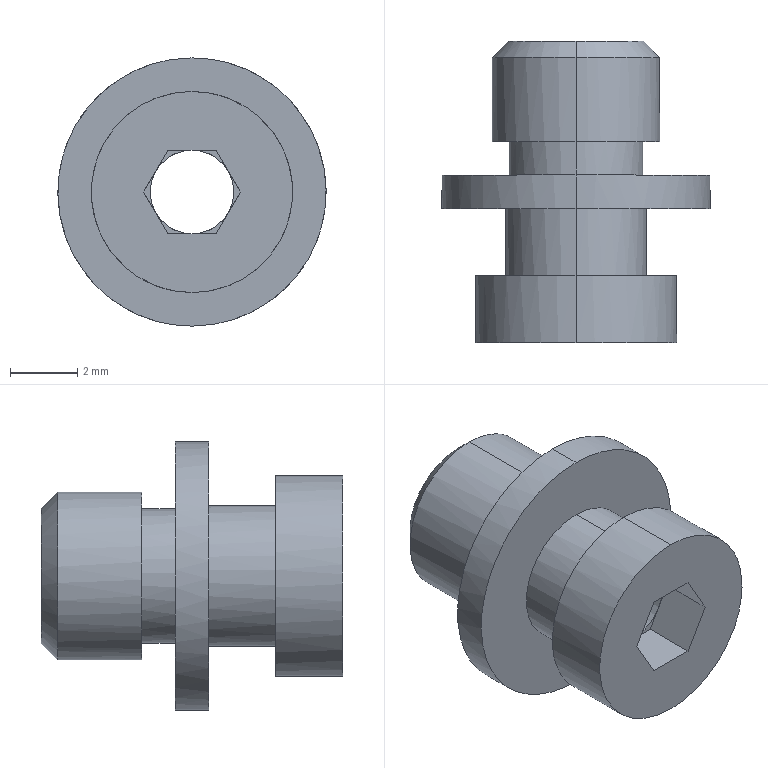Part | SolidWorks | features BaseBody 1 | 1 solid | 32 faces | box 8 x 9 x 8 mm | volume 159.238 mm3 | plane 18 | cylinder 12 | cone 2 | commonest cylinder face diameters 2.5 x2 4 x2 4.2 x2 5 x2 6 x2 8 x2
STEP:
#1=CARTESIAN_POINT('',(0.,0.,-2.1));
#2=VERTEX_POINT('',#1);
#3=CARTESIAN_POINT('',(0.,0.,2.1));
#4=VERTEX_POINT('',#3);
#5=CARTESIAN_POINT('',(0.,0.,-2.1));
#6=CARTESIAN_POINT('',(0.2749,0.,-2.1));
#7=CARTESIAN_POINT('',(0.5497,0.,-2.045));
#8=CARTESIAN_POINT('',(1.058,0.,-1.835));
#9=CARTESIAN_POINT('',(1.291,0.,-1.679));
#10=CARTESIAN_POINT('',(1.679,0.,-1.291));
#11=CARTESIAN_POINT('',(1.835,0.,-1.058));
#12=CARTESIAN_POINT('',(2.045,0.,-0.5497));
#13=CARTESIAN_POINT('',(2.1,0.,-0.2749));
#14=CARTESIAN_POINT('',(2.1,0.,0.2749));
#15=CARTESIAN_POINT('',(2.045,0.,0.5497));
#16=CARTESIAN_POINT('',(1.835,0.,1.058));
#17=CARTESIAN_POINT('',(1.679,0.,1.291));
#18=CARTESIAN_POINT('',(1.291,0.,1.679));
#19=CARTESIAN_POINT('',(1.058,0.,1.835));
#20=CARTESIAN_POINT('',(0.5497,0.,2.045));
#21=CARTESIAN_POINT('',(0.2749,0.,2.1));
#22=CARTESIAN_POINT('',(0.,0.,2.1));
#23=B_SPLINE_CURVE_WITH_KNOTS('',3,(#5,#6,#7,#8,#9,#10,#11,#12,#13,#14,#15,#16,#17,#18,#19,#20,#21,#22),.UNSPECIFIED.,.F.,.F.,(4,2,2,2,2,2,2,2,4),(0.,0.3927,0.7854,1.178,1.571,1.963,2.356,2.749,3.142),.UNSPECIFIED.);
#24=EDGE_CURVE('',#2,#4,#23,.T.);
#25=ORIENTED_EDGE('',*,*,#24,.T.);
#26=CARTESIAN_POINT('',(0.,-2.,2.1));
#27=VERTEX_POINT('',#26);
#28=CARTESIAN_POINT('',(0.,-4.,2.1));
#29=DIRECTION('',(0.,-1.,0.));
#30=VECTOR('',#29,1000.);
#31=LINE('',#28,#30);
#32=EDGE_CURVE('',#4,#27,#31,.T.);
#33=ORIENTED_EDGE('',*,*,#32,.T.);
#34=CARTESIAN_POINT('',(0.,-2.,-2.1));
#35=VERTEX_POINT('',#34);
#36=CARTESIAN_POINT('',(0.,-2.,-2.1));
#37=CARTESIAN_POINT('',(0.2785,-2.,-2.1));
#38=CARTESIAN_POINT('',(0.5464,-2.,-2.047));
#39=CARTESIAN_POINT('',(1.061,-2.,-1.834));
#40=CARTESIAN_POINT('',(1.288,-2.,-1.682));
#41=CARTESIAN_POINT('',(1.682,-2.,-1.288));
#42=CARTESIAN_POINT('',(1.834,-2.,-1.061));
#43=CARTESIAN_POINT('',(2.047,-2.,-0.5464));
#44=CARTESIAN_POINT('',(2.1,-2.,-0.2785));
#45=CARTESIAN_POINT('',(2.1,-2.,0.2785));
#46=CARTESIAN_POINT('',(2.047,-2.,0.5464));
#47=CARTESIAN_POINT('',(1.834,-2.,1.061));
#48=CARTESIAN_POINT('',(1.682,-2.,1.288));
#49=CARTESIAN_POINT('',(1.288,-2.,1.682));
#50=CARTESIAN_POINT('',(1.061,-2.,1.834));
#51=CARTESIAN_POINT('',(0.5464,-2.,2.047));
#52=CARTESIAN_POINT('',(0.2785,-2.,2.1));
#53=CARTESIAN_POINT('',(0.,-2.,2.1));
#54=B_SPLINE_CURVE_WITH_KNOTS('',3,(#36,#37,#38,#39,#40,#41,#42,#43,#44,#45,#46,#47,#48,#49,#50,#51,#52,#53),.UNSPECIFIED.,.F.,.F.,(4,2,2,2,2,2,2,2,4),(0.,0.3927,0.7854,1.178,1.571,1.963,2.356,2.749,3.142),.UNSPECIFIED.);
#55=EDGE_CURVE('',#35,#27,#54,.T.);
#56=ORIENTED_EDGE('',*,*,#55,.F.);
#57=CARTESIAN_POINT('',(0.,-4.,-2.1));
#58=DIRECTION('',(0.,-1.,0.));
#59=VECTOR('',#58,1000.);
#60=LINE('',#57,#59);
#61=EDGE_CURVE('',#2,#35,#60,.T.);
#62=ORIENTED_EDGE('',*,*,#61,.F.);
#63=EDGE_LOOP('',(#25,#33,#56,#62));
#64=FACE_OUTER_BOUND('',#63,.T.);
#65=CARTESIAN_POINT('',(0.,-4.,0.));
#66=DIRECTION('',(0.,-1.,0.));
#67=DIRECTION('',(0.,0.,-1.));
#68=AXIS2_PLACEMENT_3D('',#65,#66,#67);
#69=CYLINDRICAL_SURFACE('',#68,2.1);
#70=ADVANCED_FACE('',(#64),#69,.T.);
#71=CARTESIAN_POINT('',(0.,-2.,-3.));
#72=VERTEX_POINT('',#71);
#73=CARTESIAN_POINT('',(0.,-2.,3.));
#74=VERTEX_POINT('',#73);
#75=CARTESIAN_POINT('',(0.,-2.,-3.));
#76=CARTESIAN_POINT('',(0.3927,-2.,-3.));
#77=CARTESIAN_POINT('',(0.7852,-2.,-2.922));
#78=CARTESIAN_POINT('',(1.511,-2.,-2.621));
#79=CARTESIAN_POINT('',(1.844,-2.,-2.399));
#80=CARTESIAN_POINT('',(2.399,-2.,-1.844));
#81=CARTESIAN_POINT('',(2.621,-2.,-1.511));
#82=CARTESIAN_POINT('',(2.922,-2.,-0.7852));
#83=CARTESIAN_POINT('',(3.,-2.,-0.3927));
#84=CARTESIAN_POINT('',(3.,-2.,0.3927));
#85=CARTESIAN_POINT('',(2.922,-2.,0.7852));
#86=CARTESIAN_POINT('',(2.621,-2.,1.511));
#87=CARTESIAN_POINT('',(2.399,-2.,1.844));
#88=CARTESIAN_POINT('',(1.844,-2.,2.399));
#89=CARTESIAN_POINT('',(1.511,-2.,2.621));
#90=CARTESIAN_POINT('',(0.7852,-2.,2.922));
#91=CARTESIAN_POINT('',(0.3927,-2.,3.));
#92=CARTESIAN_POINT('',(0.,-2.,3.));
#93=B_SPLINE_CURVE_WITH_KNOTS('',3,(#75,#76,#77,#78,#79,#80,#81,#82,#83,#84,#85,#86,#87,#88,#89,#90,#91,#92),.UNSPECIFIED.,.F.,.F.,(4,2,2,2,2,2,2,2,4),(0.,0.3927,0.7854,1.178,1.571,1.963,2.356,2.749,3.142),.UNSPECIFIED.);
#94=EDGE_CURVE('',#72,#74,#93,.T.);
#95=ORIENTED_EDGE('',*,*,#94,.T.);
#96=CARTESIAN_POINT('',(0.,-4.,3.));
#97=VERTEX_POINT('',#96);
#98=CARTESIAN_POINT('',(0.,-4.,3.));
#99=DIRECTION('',(0.,-1.,0.));
#100=VECTOR('',#99,1000.);
#101=LINE('',#98,#100);
#102=EDGE_CURVE('',#74,#97,#101,.T.);
#103=ORIENTED_EDGE('',*,*,#102,.T.);
#104=CARTESIAN_POINT('',(0.,-4.,-3.));
#105=VERTEX_POINT('',#104);
#106=CARTESIAN_POINT('',(0.,-4.,-3.));
#107=CARTESIAN_POINT('',(0.3978,-4.,-3.));
#108=CARTESIAN_POINT('',(0.7805,-4.,-2.924));
#109=CARTESIAN_POINT('',(1.516,-4.,-2.619));
#110=CARTESIAN_POINT('',(1.84,-4.,-2.403));
#111=CARTESIAN_POINT('',(2.403,-4.,-1.84));
#112=CARTESIAN_POINT('',(2.619,-4.,-1.516));
#113=CARTESIAN_POINT('',(2.924,-4.,-0.7805));
#114=CARTESIAN_POINT('',(3.,-4.,-0.3978));
#115=CARTESIAN_POINT('',(3.,-4.,0.3978));
#116=CARTESIAN_POINT('',(2.924,-4.,0.7805));
#117=CARTESIAN_POINT('',(2.619,-4.,1.516));
#118=CARTESIAN_POINT('',(2.403,-4.,1.84));
#119=CARTESIAN_POINT('',(1.84,-4.,2.403));
#120=CARTESIAN_POINT('',(1.516,-4.,2.619));
#121=CARTESIAN_POINT('',(0.7805,-4.,2.924));
#122=CARTESIAN_POINT('',(0.3978,-4.,3.));
#123=CARTESIAN_POINT('',(0.,-4.,3.));
#124=B_SPLINE_CURVE_WITH_KNOTS('',3,(#106,#107,#108,#109,#110,#111,#112,#113,#114,#115,#116,#117,#118,#119,#120,#121,#122,#123),.UNSPECIFIED.,.F.,.F.,(4,2,2,2,2,2,2,2,4),(0.,0.3927,0.7854,1.178,1.571,1.963,2.356,2.749,3.142),.UNSPECIFIED.);
#125=EDGE_CURVE('',#105,#97,#124,.T.);
#126=ORIENTED_EDGE('',*,*,#125,.F.);
#127=CARTESIAN_POINT('',(0.,-4.,-3.));
#128=DIRECTION('',(0.,-1.,0.));
#129=VECTOR('',#128,1000.);
#130=LINE('',#127,#129);
#131=EDGE_CURVE('',#72,#105,#130,.T.);
#132=ORIENTED_EDGE('',*,*,#131,.F.);
#133=EDGE_LOOP('',(#95,#103,#126,#132));
#134=FACE_OUTER_BOUND('',#133,.T.);
#135=CARTESIAN_POINT('',(0.,-4.,0.));
#136=DIRECTION('',(0.,-1.,0.));
#137=DIRECTION('',(0.,0.,-1.));
#138=AXIS2_PLACEMENT_3D('',#135,#136,#137);
#139=CYLINDRICAL_SURFACE('',#138,3.);
#140=ADVANCED_FACE('',(#134),#139,.T.);
#141=CARTESIAN_POINT('',(0.,5.,-2.009));
#142=VERTEX_POINT('',#141);
#143=CARTESIAN_POINT('',(0.,5.,2.009));
#144=VERTEX_POINT('',#143);
#145=CARTESIAN_POINT('',(0.,5.,-2.009));
#146=CARTESIAN_POINT('',(0.263,5.,-2.009));
#147=CARTESIAN_POINT('',(0.526,5.,-1.957));
#148=CARTESIAN_POINT('',(1.012,5.,-1.756));
#149=CARTESIAN_POINT('',(1.235,5.,-1.607));
#150=CARTESIAN_POINT('',(1.607,5.,-1.235));
#151=CARTESIAN_POINT('',(1.756,5.,-1.012));
#152=CARTESIAN_POINT('',(1.957,5.,-0.526));
#153=CARTESIAN_POINT('',(2.009,5.,-0.263));
#154=CARTESIAN_POINT('',(2.009,5.,0.263));
#155=CARTESIAN_POINT('',(1.957,5.,0.526));
#156=CARTESIAN_POINT('',(1.756,5.,1.012));
#157=CARTESIAN_POINT('',(1.607,5.,1.235));
#158=CARTESIAN_POINT('',(1.235,5.,1.607));
#159=CARTESIAN_POINT('',(1.012,5.,1.756));
#160=CARTESIAN_POINT('',(0.526,5.,1.957));
#161=CARTESIAN_POINT('',(0.263,5.,2.009));
#162=CARTESIAN_POINT('',(0.,5.,2.009));
#163=B_SPLINE_CURVE_WITH_KNOTS('',3,(#145,#146,#147,#148,#149,#150,#151,#152,#153,#154,#155,#156,#157,#158,#159,#160,#161,#162),.UNSPECIFIED.,.F.,.F.,(4,2,2,2,2,2,2,2,4),(0.,0.3927,0.7854,1.178,1.571,1.963,2.356,2.749,3.142),.UNSPECIFIED.);
#164=EDGE_CURVE('',#142,#144,#163,.T.);
#165=ORIENTED_EDGE('',*,*,#164,.T.);
#166=CARTESIAN_POINT('',(0.,4.509,2.5));
#167=VERTEX_POINT('',#166);
#168=CARTESIAN_POINT('',(0.,4.509,2.5));
#169=DIRECTION('',(0.,-0.7071,0.7071));
#170=VECTOR('',#169,1000.);
#171=LINE('',#168,#170);
#172=EDGE_CURVE('',#144,#167,#171,.T.);
#173=ORIENTED_EDGE('',*,*,#172,.T.);
#174=CARTESIAN_POINT('',(0.,4.509,-2.5));
#175=VERTEX_POINT('',#174);
#176=CARTESIAN_POINT('',(0.,4.509,-2.5));
#177=CARTESIAN_POINT('',(0.3272,4.509,-2.5));
#178=CARTESIAN_POINT('',(0.6544,4.509,-2.435));
#179=CARTESIAN_POINT('',(1.259,4.509,-2.184));
#180=CARTESIAN_POINT('',(1.536,4.51,-1.999));
#181=CARTESIAN_POINT('',(1.999,4.509,-1.536));
#182=CARTESIAN_POINT('',(2.184,4.51,-1.259));
#183=CARTESIAN_POINT('',(2.435,4.509,-0.6544));
#184=CARTESIAN_POINT('',(2.5,4.51,-0.3272));
#185=CARTESIAN_POINT('',(2.5,4.509,0.3272));
#186=CARTESIAN_POINT('',(2.435,4.509,0.6544));
#187=CARTESIAN_POINT('',(2.184,4.509,1.259));
#188=CARTESIAN_POINT('',(1.999,4.509,1.536));
#189=CARTESIAN_POINT('',(1.536,4.509,1.999));
#190=CARTESIAN_POINT('',(1.259,4.509,2.184));
#191=CARTESIAN_POINT('',(0.6544,4.51,2.435));
#192=CARTESIAN_POINT('',(0.3272,4.51,2.5));
#193=CARTESIAN_POINT('',(0.,4.509,2.5));
#194=B_SPLINE_CURVE_WITH_KNOTS('',3,(#176,#177,#178,#179,#180,#181,#182,#183,#184,#185,#186,#187,#188,#189,#190,#191,#192,#193),.UNSPECIFIED.,.F.,.F.,(4,2,2,2,2,2,2,2,4),(0.,0.3927,0.7854,1.178,1.571,1.963,2.356,2.749,3.142),.UNSPECIFIED.);
#195=EDGE_CURVE('',#175,#167,#194,.T.);
#196=ORIENTED_EDGE('',*,*,#195,.F.);
#197=CARTESIAN_POINT('',(0.,4.509,-2.5));
#198=DIRECTION('',(0.,-0.7071,-0.7071));
#199=VECTOR('',#198,1000.);
#200=LINE('',#197,#199);
#201=EDGE_CURVE('',#142,#175,#200,.T.);
#202=ORIENTED_EDGE('',*,*,#201,.F.);
#203=EDGE_LOOP('',(#165,#173,#196,#202));
#204=FACE_OUTER_BOUND('',#203,.T.);
#205=CARTESIAN_POINT('',(0.,4.509,0.));
#206=DIRECTION('',(0.,-1.,0.));
#207=DIRECTION('',(0.,0.,-1.));
#208=AXIS2_PLACEMENT_3D('',#205,#206,#207);
#209=CONICAL_SURFACE('',#208,2.5,0.7854);
#210=ADVANCED_FACE('',(#204),#209,.T.);
#211=ORIENTED_EDGE('',*,*,#195,.T.);
#212=CARTESIAN_POINT('',(0.,2.,2.5));
#213=VERTEX_POINT('',#212);
#214=CARTESIAN_POINT('',(0.,0.,2.5));
#215=DIRECTION('',(0.,-1.,0.));
#216=VECTOR('',#215,1000.);
#217=LINE('',#214,#216);
#218=EDGE_CURVE('',#167,#213,#217,.T.);
#219=ORIENTED_EDGE('',*,*,#218,.T.);
#220=CARTESIAN_POINT('',(0.,2.,-2.5));
#221=VERTEX_POINT('',#220);
#222=CARTESIAN_POINT('',(0.,2.,-2.5));
#223=CARTESIAN_POINT('',(0.3315,2.,-2.5));
#224=CARTESIAN_POINT('',(0.6504,2.,-2.437));
#225=CARTESIAN_POINT('',(1.263,2.,-2.183));
#226=CARTESIAN_POINT('',(1.533,2.,-2.002));
#227=CARTESIAN_POINT('',(2.002,2.,-1.533));
#228=CARTESIAN_POINT('',(2.183,2.,-1.263));
#229=CARTESIAN_POINT('',(2.437,2.,-0.6504));
#230=CARTESIAN_POINT('',(2.5,2.,-0.3315));
#231=CARTESIAN_POINT('',(2.5,2.,0.3315));
#232=CARTESIAN_POINT('',(2.437,2.,0.6504));
#233=CARTESIAN_POINT('',(2.183,2.,1.263));
#234=CARTESIAN_POINT('',(2.002,2.,1.533));
#235=CARTESIAN_POINT('',(1.533,2.,2.002));
#236=CARTESIAN_POINT('',(1.263,2.,2.183));
#237=CARTESIAN_POINT('',(0.6504,2.,2.437));
#238=CARTESIAN_POINT('',(0.3315,2.,2.5));
#239=CARTESIAN_POINT('',(0.,2.,2.5));
#240=B_SPLINE_CURVE_WITH_KNOTS('',3,(#222,#223,#224,#225,#226,#227,#228,#229,#230,#231,#232,#233,#234,#235,#236,#237,#238,#239),.UNSPECIFIED.,.F.,.F.,(4,2,2,2,2,2,2,2,4),(0.,0.3927,0.7854,1.178,1.571,1.963,2.356,2.749,3.142),.UNSPECIFIED.);
#241=EDGE_CURVE('',#221,#213,#240,.T.);
#242=ORIENTED_EDGE('',*,*,#241,.F.);
#243=CARTESIAN_POINT('',(0.,0.,-2.5));
#244=DIRECTION('',(0.,-1.,0.));
#245=VECTOR('',#244,1000.);
#246=LINE('',#243,#245);
#247=EDGE_CURVE('',#175,#221,#246,.T.);
#248=ORIENTED_EDGE('',*,*,#247,.F.);
#249=EDGE_LOOP('',(#211,#219,#242,#248));
#250=FACE_OUTER_BOUND('',#249,.T.);
#251=CARTESIAN_POINT('',(0.,0.,0.));
#252=DIRECTION('',(0.,-1.,0.));
#253=DIRECTION('',(0.,0.,-1.));
#254=AXIS2_PLACEMENT_3D('',#251,#252,#253);
#255=CYLINDRICAL_SURFACE('',#254,2.5);
#256=ADVANCED_FACE('',(#250),#255,.T.);
#257=CARTESIAN_POINT('',(0.,2.,-2.));
#258=VERTEX_POINT('',#257);
#259=CARTESIAN_POINT('',(0.,2.,2.));
#260=VERTEX_POINT('',#259);
#261=CARTESIAN_POINT('',(0.,2.,-2.));
#262=CARTESIAN_POINT('',(0.2618,2.,-2.));
#263=CARTESIAN_POINT('',(0.5235,2.,-1.948));
#264=CARTESIAN_POINT('',(1.007,2.,-1.748));
#265=CARTESIAN_POINT('',(1.229,2.,-1.599));
#266=CARTESIAN_POINT('',(1.599,2.,-1.229));
#267=CARTESIAN_POINT('',(1.748,2.,-1.007));
#268=CARTESIAN_POINT('',(1.948,2.,-0.5235));
#269=CARTESIAN_POINT('',(2.,2.,-0.2618));
#270=CARTESIAN_POINT('',(2.,2.,0.2618));
#271=CARTESIAN_POINT('',(1.948,2.,0.5235));
#272=CARTESIAN_POINT('',(1.748,2.,1.007));
#273=CARTESIAN_POINT('',(1.599,2.,1.229));
#274=CARTESIAN_POINT('',(1.229,2.,1.599));
#275=CARTESIAN_POINT('',(1.007,2.,1.748));
#276=CARTESIAN_POINT('',(0.5235,2.,1.948));
#277=CARTESIAN_POINT('',(0.2618,2.,2.));
#278=CARTESIAN_POINT('',(0.,2.,2.));
#279=B_SPLINE_CURVE_WITH_KNOTS('',3,(#261,#262,#263,#264,#265,#266,#267,#268,#269,#270,#271,#272,#273,#274,#275,#276,#277,#278),.UNSPECIFIED.,.F.,.F.,(4,2,2,2,2,2,2,2,4),(0.,0.3927,0.7854,1.178,1.571,1.963,2.356,2.749,3.142),.UNSPECIFIED.);
#280=EDGE_CURVE('',#258,#260,#279,.T.);
#281=ORIENTED_EDGE('',*,*,#280,.T.);
#282=CARTESIAN_POINT('',(0.,1.,2.));
#283=VERTEX_POINT('',#282);
#284=CARTESIAN_POINT('',(0.,0.,2.));
#285=DIRECTION('',(0.,-1.,0.));
#286=VECTOR('',#285,1000.);
#287=LINE('',#284,#286);
#288=EDGE_CURVE('',#260,#283,#287,.T.);
#289=ORIENTED_EDGE('',*,*,#288,.T.);
#290=CARTESIAN_POINT('',(0.,1.,-2.));
#291=VERTEX_POINT('',#290);
#292=CARTESIAN_POINT('',(0.,1.,-2.));
#293=CARTESIAN_POINT('',(0.2652,1.,-2.));
#294=CARTESIAN_POINT('',(0.5203,1.,-1.949));
#295=CARTESIAN_POINT('',(1.01,1.,-1.746));
#296=CARTESIAN_POINT('',(1.227,1.,-1.602));
#297=CARTESIAN_POINT('',(1.602,1.,-1.227));
#298=CARTESIAN_POINT('',(1.746,1.,-1.01));
#299=CARTESIAN_POINT('',(1.949,1.,-0.5203));
#300=CARTESIAN_POINT('',(2.,1.,-0.2652));
#301=CARTESIAN_POINT('',(2.,1.,0.2652));
#302=CARTESIAN_POINT('',(1.949,1.,0.5203));
#303=CARTESIAN_POINT('',(1.746,1.,1.01));
#304=CARTESIAN_POINT('',(1.602,1.,1.227));
#305=CARTESIAN_POINT('',(1.227,1.,1.602));
#306=CARTESIAN_POINT('',(1.01,1.,1.746));
#307=CARTESIAN_POINT('',(0.5203,1.,1.949));
#308=CARTESIAN_POINT('',(0.2652,1.,2.));
#309=CARTESIAN_POINT('',(0.,1.,2.));
#310=B_SPLINE_CURVE_WITH_KNOTS('',3,(#292,#293,#294,#295,#296,#297,#298,#299,#300,#301,#302,#303,#304,#305,#306,#307,#308,#309),.UNSPECIFIED.,.F.,.F.,(4,2,2,2,2,2,2,2,4),(0.,0.3927,0.7854,1.178,1.571,1.963,2.356,2.749,3.142),.UNSPECIFIED.);
#311=EDGE_CURVE('',#291,#283,#310,.T.);
#312=ORIENTED_EDGE('',*,*,#311,.F.);
#313=CARTESIAN_POINT('',(0.,0.,-2.));
#314=DIRECTION('',(0.,-1.,0.));
#315=VECTOR('',#314,1000.);
#316=LINE('',#313,#315);
#317=EDGE_CURVE('',#258,#291,#316,.T.);
#318=ORIENTED_EDGE('',*,*,#317,.F.);
#319=EDGE_LOOP('',(#281,#289,#312,#318));
#320=FACE_OUTER_BOUND('',#319,.T.);
#321=CARTESIAN_POINT('',(0.,0.,0.));
#322=DIRECTION('',(0.,-1.,0.));
#323=DIRECTION('',(0.,0.,-1.));
#324=AXIS2_PLACEMENT_3D('',#321,#322,#323);
#325=CYLINDRICAL_SURFACE('',#324,2.);
#326=ADVANCED_FACE('',(#320),#325,.T.);
#327=CARTESIAN_POINT('',(0.,1.,-4.));
#328=VERTEX_POINT('',#327);
#329=CARTESIAN_POINT('',(0.,1.,4.));
#330=VERTEX_POINT('',#329);
#331=CARTESIAN_POINT('',(0.,1.,-4.));
#332=CARTESIAN_POINT('',(0.5236,1.,-4.));
#333=CARTESIAN_POINT('',(1.047,1.,-3.896));
#334=CARTESIAN_POINT('',(2.014,1.,-3.495));
#335=CARTESIAN_POINT('',(2.458,1.,-3.199));
#336=CARTESIAN_POINT('',(3.199,1.,-2.458));
#337=CARTESIAN_POINT('',(3.495,1.,-2.014));
#338=CARTESIAN_POINT('',(3.896,1.,-1.047));
#339=CARTESIAN_POINT('',(4.,1.,-0.5236));
#340=CARTESIAN_POINT('',(4.,1.,0.5236));
#341=CARTESIAN_POINT('',(3.896,1.,1.047));
#342=CARTESIAN_POINT('',(3.495,1.,2.014));
#343=CARTESIAN_POINT('',(3.199,1.,2.458));
#344=CARTESIAN_POINT('',(2.458,1.,3.199));
#345=CARTESIAN_POINT('',(2.014,1.,3.495));
#346=CARTESIAN_POINT('',(1.047,1.,3.896));
#347=CARTESIAN_POINT('',(0.5236,1.,4.));
#348=CARTESIAN_POINT('',(0.,1.,4.));
#349=B_SPLINE_CURVE_WITH_KNOTS('',3,(#331,#332,#333,#334,#335,#336,#337,#338,#339,#340,#341,#342,#343,#344,#345,#346,#347,#348),.UNSPECIFIED.,.F.,.F.,(4,2,2,2,2,2,2,2,4),(0.,0.3927,0.7854,1.178,1.571,1.963,2.356,2.749,3.142),.UNSPECIFIED.);
#350=EDGE_CURVE('',#328,#330,#349,.T.);
#351=ORIENTED_EDGE('',*,*,#350,.T.);
#352=CARTESIAN_POINT('',(0.,0.,4.));
#353=VERTEX_POINT('',#352);
#354=CARTESIAN_POINT('',(0.,0.,4.));
#355=DIRECTION('',(0.,-1.,0.));
#356=VECTOR('',#355,1000.);
#357=LINE('',#354,#356);
#358=EDGE_CURVE('',#330,#353,#357,.T.);
#359=ORIENTED_EDGE('',*,*,#358,.T.);
#360=CARTESIAN_POINT('',(0.,0.,-4.));
#361=VERTEX_POINT('',#360);
#362=CARTESIAN_POINT('',(0.,0.,-4.));
#363=CARTESIAN_POINT('',(0.5304,0.,-4.));
#364=CARTESIAN_POINT('',(1.041,0.,-3.899));
#365=CARTESIAN_POINT('',(2.021,0.,-3.493));
#366=CARTESIAN_POINT('',(2.453,0.,-3.203));
#367=CARTESIAN_POINT('',(3.203,0.,-2.453));
#368=CARTESIAN_POINT('',(3.493,0.,-2.021));
#369=CARTESIAN_POINT('',(3.899,0.,-1.041));
#370=CARTESIAN_POINT('',(4.,0.,-0.5304));
#371=CARTESIAN_POINT('',(4.,0.,0.5304));
#372=CARTESIAN_POINT('',(3.899,0.,1.041));
#373=CARTESIAN_POINT('',(3.493,0.,2.021));
#374=CARTESIAN_POINT('',(3.203,0.,2.453));
#375=CARTESIAN_POINT('',(2.453,0.,3.203));
#376=CARTESIAN_POINT('',(2.021,0.,3.493));
#377=CARTESIAN_POINT('',(1.041,0.,3.899));
#378=CARTESIAN_POINT('',(0.5304,0.,4.));
#379=CARTESIAN_POINT('',(0.,0.,4.));
#380=B_SPLINE_CURVE_WITH_KNOTS('',3,(#362,#363,#364,#365,#366,#367,#368,#369,#370,#371,#372,#373,#374,#375,#376,#377,#378,#379),.UNSPECIFIED.,.F.,.F.,(4,2,2,2,2,2,2,2,4),(0.,0.3927,0.7854,1.178,1.571,1.963,2.356,2.749,3.142),.UNSPECIFIED.);
#381=EDGE_CURVE('',#361,#353,#380,.T.);
#382=ORIENTED_EDGE('',*,*,#381,.F.);
#383=CARTESIAN_POINT('',(0.,0.,-4.));
#384=DIRECTION('',(0.,-1.,0.));
#385=VECTOR('',#384,1000.);
#386=LINE('',#383,#385);
#387=EDGE_CURVE('',#328,#361,#386,.T.);
#388=ORIENTED_EDGE('',*,*,#387,.F.);
#389=EDGE_LOOP('',(#351,#359,#382,#388));
#390=FACE_OUTER_BOUND('',#389,.T.);
#391=CARTESIAN_POINT('',(0.,0.,0.));
#392=DIRECTION('',(0.,-1.,0.));
#393=DIRECTION('',(0.,0.,-1.));
#394=AXIS2_PLACEMENT_3D('',#391,#392,#393);
#395=CYLINDRICAL_SURFACE('',#394,4.);
#396=ADVANCED_FACE('',(#390),#395,.T.);
#397=CARTESIAN_POINT('',(0.,5.,1.25));
#398=VERTEX_POINT('',#397);
#399=CARTESIAN_POINT('',(0.,5.,-1.25));
#400=VERTEX_POINT('',#399);
#401=CARTESIAN_POINT('',(0.,5.,1.25));
#402=CARTESIAN_POINT('',(-0.1658,5.,1.25));
#403=CARTESIAN_POINT('',(-0.3252,5.,1.218));
#404=CARTESIAN_POINT('',(-0.6315,5.,1.091));
#405=CARTESIAN_POINT('',(-0.7667,5.,1.001));
#406=CARTESIAN_POINT('',(-1.001,5.,0.7667));
#407=CARTESIAN_POINT('',(-1.091,5.,0.6315));
#408=CARTESIAN_POINT('',(-1.218,5.,0.3252));
#409=CARTESIAN_POINT('',(-1.25,5.,0.1658));
#410=CARTESIAN_POINT('',(-1.25,5.,-0.1658));
#411=CARTESIAN_POINT('',(-1.218,5.,-0.3252));
#412=CARTESIAN_POINT('',(-1.091,5.,-0.6315));
#413=CARTESIAN_POINT('',(-1.001,5.,-0.7667));
#414=CARTESIAN_POINT('',(-0.7667,5.,-1.001));
#415=CARTESIAN_POINT('',(-0.6315,5.,-1.091));
#416=CARTESIAN_POINT('',(-0.3252,5.,-1.218));
#417=CARTESIAN_POINT('',(-0.1658,5.,-1.25));
#418=CARTESIAN_POINT('',(0.,5.,-1.25));
#419=B_SPLINE_CURVE_WITH_KNOTS('',3,(#401,#402,#403,#404,#405,#406,#407,#408,#409,#410,#411,#412,#413,#414,#415,#416,#417,#418),.UNSPECIFIED.,.F.,.F.,(4,2,2,2,2,2,2,2,4),(3.142,3.534,3.927,4.32,4.712,5.105,5.498,5.89,6.283),.UNSPECIFIED.);
#420=EDGE_CURVE('',#398,#400,#419,.T.);
#421=ORIENTED_EDGE('',*,*,#420,.F.);
#422=CARTESIAN_POINT('',(0.,-2.4,1.25));
#423=VERTEX_POINT('',#422);
#424=CARTESIAN_POINT('',(0.,0.,1.25));
#425=DIRECTION('',(0.,-1.,0.));
#426=VECTOR('',#425,1000.);
#427=LINE('',#424,#426);
#428=EDGE_CURVE('',#398,#423,#427,.T.);
#429=ORIENTED_EDGE('',*,*,#428,.T.);
#430=CARTESIAN_POINT('',(-1.083,-2.4,0.625));
#431=VERTEX_POINT('',#430);
#432=CARTESIAN_POINT('',(0.,-2.4,0.));
#433=DIRECTION('',(0.,-1.,0.));
#434=DIRECTION('',(0.,0.,1.));
#435=AXIS2_PLACEMENT_3D('',#432,#433,#434);
#436=CIRCLE('',#435,1.25);
#437=EDGE_CURVE('',#423,#431,#436,.T.);
#438=ORIENTED_EDGE('',*,*,#437,.T.);
#439=CARTESIAN_POINT('',(-1.083,-2.4,-0.625));
#440=VERTEX_POINT('',#439);
#441=CARTESIAN_POINT('',(0.,-2.4,0.));
#442=DIRECTION('',(0.,-1.,0.));
#443=DIRECTION('',(-0.866,0.,0.5));
#444=AXIS2_PLACEMENT_3D('',#441,#442,#443);
#445=CIRCLE('',#444,1.25);
#446=EDGE_CURVE('',#431,#440,#445,.T.);
#447=ORIENTED_EDGE('',*,*,#446,.T.);
#448=CARTESIAN_POINT('',(0.,-2.4,-1.25));
#449=VERTEX_POINT('',#448);
#450=CARTESIAN_POINT('',(0.,-2.4,0.));
#451=DIRECTION('',(0.,-1.,0.));
#452=DIRECTION('',(-0.866,0.,-0.5));
#453=AXIS2_PLACEMENT_3D('',#450,#451,#452);
#454=CIRCLE('',#453,1.25);
#455=EDGE_CURVE('',#440,#449,#454,.T.);
#456=ORIENTED_EDGE('',*,*,#455,.T.);
#457=CARTESIAN_POINT('',(0.,0.,-1.25));
#458=DIRECTION('',(0.,-1.,0.));
#459=VECTOR('',#458,1000.);
#460=LINE('',#457,#459);
#461=EDGE_CURVE('',#400,#449,#460,.T.);
#462=ORIENTED_EDGE('',*,*,#461,.F.);
#463=EDGE_LOOP('',(#421,#429,#438,#447,#456,#462));
#464=FACE_OUTER_BOUND('',#463,.T.);
#465=CARTESIAN_POINT('',(0.,0.,0.));
#466=DIRECTION('',(0.,-1.,0.));
#467=DIRECTION('',(0.,0.,-1.));
#468=AXIS2_PLACEMENT_3D('',#465,#466,#467);
#469=CYLINDRICAL_SURFACE('',#468,1.25);
#470=ADVANCED_FACE('',(#464),#469,.F.);
#471=ORIENTED_EDGE('',*,*,#428,.F.);
#472=CARTESIAN_POINT('',(0.,5.,-1.25));
#473=CARTESIAN_POINT('',(0.1658,5.,-1.25));
#474=CARTESIAN_POINT('',(0.3252,5.,-1.218));
#475=CARTESIAN_POINT('',(0.6315,5.,-1.091));
#476=CARTESIAN_POINT('',(0.7667,5.,-1.001));
#477=CARTESIAN_POINT('',(1.001,5.,-0.7667));
#478=CARTESIAN_POINT('',(1.091,5.,-0.6315));
#479=CARTESIAN_POINT('',(1.218,5.,-0.3252));
#480=CARTESIAN_POINT('',(1.25,5.,-0.1658));
#481=CARTESIAN_POINT('',(1.25,5.,0.1658));
#482=CARTESIAN_POINT('',(1.218,5.,0.3252));
#483=CARTESIAN_POINT('',(1.091,5.,0.6315));
#484=CARTESIAN_POINT('',(1.001,5.,0.7667));
#485=CARTESIAN_POINT('',(0.7667,5.,1.001));
#486=CARTESIAN_POINT('',(0.6315,5.,1.091));
#487=CARTESIAN_POINT('',(0.3252,5.,1.218));
#488=CARTESIAN_POINT('',(0.1658,5.,1.25));
#489=CARTESIAN_POINT('',(0.,5.,1.25));
#490=B_SPLINE_CURVE_WITH_KNOTS('',3,(#472,#473,#474,#475,#476,#477,#478,#479,#480,#481,#482,#483,#484,#485,#486,#487,#488,#489),.UNSPECIFIED.,.F.,.F.,(4,2,2,2,2,2,2,2,4),(0.,0.3927,0.7854,1.178,1.571,1.963,2.356,2.749,3.142),.UNSPECIFIED.);
#491=EDGE_CURVE('',#400,#398,#490,.T.);
#492=ORIENTED_EDGE('',*,*,#491,.F.);
#493=ORIENTED_EDGE('',*,*,#461,.T.);
#494=CARTESIAN_POINT('',(1.083,-2.4,-0.625));
#495=VERTEX_POINT('',#494);
#496=CARTESIAN_POINT('',(0.,-2.4,0.));
#497=DIRECTION('',(0.,-1.,0.));
#498=DIRECTION('',(0.,0.,-1.));
#499=AXIS2_PLACEMENT_3D('',#496,#497,#498);
#500=CIRCLE('',#499,1.25);
#501=EDGE_CURVE('',#449,#495,#500,.T.);
#502=ORIENTED_EDGE('',*,*,#501,.T.);
#503=CARTESIAN_POINT('',(1.083,-2.4,0.625));
#504=VERTEX_POINT('',#503);
#505=CARTESIAN_POINT('',(0.,-2.4,0.));
#506=DIRECTION('',(0.,-1.,0.));
#507=DIRECTION('',(0.866,0.,-0.5));
#508=AXIS2_PLACEMENT_3D('',#505,#506,#507);
#509=CIRCLE('',#508,1.25);
#510=EDGE_CURVE('',#495,#504,#509,.T.);
#511=ORIENTED_EDGE('',*,*,#510,.T.);
#512=CARTESIAN_POINT('',(0.,-2.4,0.));
#513=DIRECTION('',(0.,-1.,0.));
#514=DIRECTION('',(0.866,0.,0.5));
#515=AXIS2_PLACEMENT_3D('',#512,#513,#514);
#516=CIRCLE('',#515,1.25);
#517=EDGE_CURVE('',#504,#423,#516,.T.);
#518=ORIENTED_EDGE('',*,*,#517,.T.);
#519=EDGE_LOOP('',(#471,#492,#493,#502,#511,#518));
#520=FACE_OUTER_BOUND('',#519,.T.);
#521=CARTESIAN_POINT('',(0.,0.,0.));
#522=DIRECTION('',(0.,-1.,0.));
#523=DIRECTION('',(0.,0.,-1.));
#524=AXIS2_PLACEMENT_3D('',#521,#522,#523);
#525=CYLINDRICAL_SURFACE('',#524,1.25);
#526=ADVANCED_FACE('',(#520),#525,.F.);
#527=ORIENTED_EDGE('',*,*,#491,.T.);
#528=ORIENTED_EDGE('',*,*,#420,.T.);
#529=EDGE_LOOP('',(#527,#528));
#530=FACE_BOUND('',#529,.T.);
#531=ORIENTED_EDGE('',*,*,#164,.F.);
#532=CARTESIAN_POINT('',(0.,5.,2.009));
#533=CARTESIAN_POINT('',(-0.263,5.,2.009));
#534=CARTESIAN_POINT('',(-0.526,5.,1.957));
#535=CARTESIAN_POINT('',(-1.012,5.,1.756));
#536=CARTESIAN_POINT('',(-1.235,5.,1.607));
#537=CARTESIAN_POINT('',(-1.607,5.,1.235));
#538=CARTESIAN_POINT('',(-1.756,5.,1.012));
#539=CARTESIAN_POINT('',(-1.957,5.,0.526));
#540=CARTESIAN_POINT('',(-2.009,5.,0.263));
#541=CARTESIAN_POINT('',(-2.009,5.,-0.263));
#542=CARTESIAN_POINT('',(-1.957,5.,-0.526));
#543=CARTESIAN_POINT('',(-1.756,5.,-1.012));
#544=CARTESIAN_POINT('',(-1.607,5.,-1.235));
#545=CARTESIAN_POINT('',(-1.235,5.,-1.607));
#546=CARTESIAN_POINT('',(-1.012,5.,-1.756));
#547=CARTESIAN_POINT('',(-0.526,5.,-1.957));
#548=CARTESIAN_POINT('',(-0.263,5.,-2.009));
#549=CARTESIAN_POINT('',(0.,5.,-2.009));
#550=B_SPLINE_CURVE_WITH_KNOTS('',3,(#532,#533,#534,#535,#536,#537,#538,#539,#540,#541,#542,#543,#544,#545,#546,#547,#548,#549),.UNSPECIFIED.,.F.,.F.,(4,2,2,2,2,2,2,2,4),(3.142,3.534,3.927,4.32,4.712,5.105,5.498,5.89,6.283),.UNSPECIFIED.);
#551=EDGE_CURVE('',#144,#142,#550,.T.);
#552=ORIENTED_EDGE('',*,*,#551,.F.);
#553=EDGE_LOOP('',(#531,#552));
#554=FACE_OUTER_BOUND('',#553,.T.);
#555=CARTESIAN_POINT('',(2.009,5.,0.));
#556=DIRECTION('',(0.,1.,0.));
#557=DIRECTION('',(0.,0.,1.));
#558=AXIS2_PLACEMENT_3D('',#555,#556,#557);
#559=PLANE('',#558);
#560=ADVANCED_FACE('',(#530,#554),#559,.T.);
#561=ORIENTED_EDGE('',*,*,#381,.T.);
#562=CARTESIAN_POINT('',(0.,0.,4.));
#563=CARTESIAN_POINT('',(-0.5304,0.,4.));
#564=CARTESIAN_POINT('',(-1.041,0.,3.899));
#565=CARTESIAN_POINT('',(-2.021,0.,3.493));
#566=CARTESIAN_POINT('',(-2.453,0.,3.203));
#567=CARTESIAN_POINT('',(-3.203,0.,2.453));
#568=CARTESIAN_POINT('',(-3.493,0.,2.021));
#569=CARTESIAN_POINT('',(-3.899,0.,1.041));
#570=CARTESIAN_POINT('',(-4.,0.,0.5304));
#571=CARTESIAN_POINT('',(-4.,0.,-0.5304));
#572=CARTESIAN_POINT('',(-3.899,0.,-1.041));
#573=CARTESIAN_POINT('',(-3.493,0.,-2.021));
#574=CARTESIAN_POINT('',(-3.203,0.,-2.453));
#575=CARTESIAN_POINT('',(-2.453,0.,-3.203));
#576=CARTESIAN_POINT('',(-2.021,0.,-3.493));
#577=CARTESIAN_POINT('',(-1.041,0.,-3.899));
#578=CARTESIAN_POINT('',(-0.5304,0.,-4.));
#579=CARTESIAN_POINT('',(0.,0.,-4.));
#580=B_SPLINE_CURVE_WITH_KNOTS('',3,(#562,#563,#564,#565,#566,#567,#568,#569,#570,#571,#572,#573,#574,#575,#576,#577,#578,#579),.UNSPECIFIED.,.F.,.F.,(4,2,2,2,2,2,2,2,4),(3.142,3.534,3.927,4.32,4.712,5.105,5.498,5.89,6.283),.UNSPECIFIED.);
#581=EDGE_CURVE('',#353,#361,#580,.T.);
#582=ORIENTED_EDGE('',*,*,#581,.T.);
#583=EDGE_LOOP('',(#561,#582));
#584=FACE_OUTER_BOUND('',#583,.T.);
#585=ORIENTED_EDGE('',*,*,#24,.F.);
#586=CARTESIAN_POINT('',(0.,0.,2.1));
#587=CARTESIAN_POINT('',(-0.2749,0.,2.1));
#588=CARTESIAN_POINT('',(-0.5497,0.,2.045));
#589=CARTESIAN_POINT('',(-1.058,0.,1.835));
#590=CARTESIAN_POINT('',(-1.291,0.,1.679));
#591=CARTESIAN_POINT('',(-1.679,0.,1.291));
#592=CARTESIAN_POINT('',(-1.835,0.,1.058));
#593=CARTESIAN_POINT('',(-2.045,0.,0.5497));
#594=CARTESIAN_POINT('',(-2.1,0.,0.2749));
#595=CARTESIAN_POINT('',(-2.1,0.,-0.2749));
#596=CARTESIAN_POINT('',(-2.045,0.,-0.5497));
#597=CARTESIAN_POINT('',(-1.835,0.,-1.058));
#598=CARTESIAN_POINT('',(-1.679,0.,-1.291));
#599=CARTESIAN_POINT('',(-1.291,0.,-1.679));
#600=CARTESIAN_POINT('',(-1.058,0.,-1.835));
#601=CARTESIAN_POINT('',(-0.5497,0.,-2.045));
#602=CARTESIAN_POINT('',(-0.2749,0.,-2.1));
#603=CARTESIAN_POINT('',(0.,0.,-2.1));
#604=B_SPLINE_CURVE_WITH_KNOTS('',3,(#586,#587,#588,#589,#590,#591,#592,#593,#594,#595,#596,#597,#598,#599,#600,#601,#602,#603),.UNSPECIFIED.,.F.,.F.,(4,2,2,2,2,2,2,2,4),(3.142,3.534,3.927,4.32,4.712,5.105,5.498,5.89,6.283),.UNSPECIFIED.);
#605=EDGE_CURVE('',#4,#2,#604,.T.);
#606=ORIENTED_EDGE('',*,*,#605,.F.);
#607=EDGE_LOOP('',(#585,#606));
#608=FACE_BOUND('',#607,.T.);
#609=CARTESIAN_POINT('',(1.25,0.,0.));
#610=DIRECTION('',(0.,-1.,0.));
#611=DIRECTION('',(0.,0.,-1.));
#612=AXIS2_PLACEMENT_3D('',#609,#610,#611);
#613=PLANE('',#612);
#614=ADVANCED_FACE('',(#584,#608),#613,.T.);
#615=ORIENTED_EDGE('',*,*,#358,.F.);
#616=CARTESIAN_POINT('',(0.,1.,4.));
#617=CARTESIAN_POINT('',(-0.5236,1.,4.));
#618=CARTESIAN_POINT('',(-1.047,1.,3.896));
#619=CARTESIAN_POINT('',(-2.014,1.,3.495));
#620=CARTESIAN_POINT('',(-2.458,1.,3.199));
#621=CARTESIAN_POINT('',(-3.199,1.,2.458));
#622=CARTESIAN_POINT('',(-3.495,1.,2.014));
#623=CARTESIAN_POINT('',(-3.896,1.,1.047));
#624=CARTESIAN_POINT('',(-4.,1.,0.5236));
#625=CARTESIAN_POINT('',(-4.,1.,-0.5236));
#626=CARTESIAN_POINT('',(-3.896,1.,-1.047));
#627=CARTESIAN_POINT('',(-3.495,1.,-2.014));
#628=CARTESIAN_POINT('',(-3.199,1.,-2.458));
#629=CARTESIAN_POINT('',(-2.458,1.,-3.199));
#630=CARTESIAN_POINT('',(-2.014,1.,-3.495));
#631=CARTESIAN_POINT('',(-1.047,1.,-3.896));
#632=CARTESIAN_POINT('',(-0.5236,1.,-4.));
#633=CARTESIAN_POINT('',(0.,1.,-4.));
#634=B_SPLINE_CURVE_WITH_KNOTS('',3,(#616,#617,#618,#619,#620,#621,#622,#623,#624,#625,#626,#627,#628,#629,#630,#631,#632,#633),.UNSPECIFIED.,.F.,.F.,(4,2,2,2,2,2,2,2,4),(3.142,3.534,3.927,4.32,4.712,5.105,5.498,5.89,6.283),.UNSPECIFIED.);
#635=EDGE_CURVE('',#330,#328,#634,.T.);
#636=ORIENTED_EDGE('',*,*,#635,.T.);
#637=ORIENTED_EDGE('',*,*,#387,.T.);
#638=ORIENTED_EDGE('',*,*,#581,.F.);
#639=EDGE_LOOP('',(#615,#636,#637,#638));
#640=FACE_OUTER_BOUND('',#639,.T.);
#641=CARTESIAN_POINT('',(0.,0.,0.));
#642=DIRECTION('',(0.,-1.,0.));
#643=DIRECTION('',(0.,0.,-1.));
#644=AXIS2_PLACEMENT_3D('',#641,#642,#643);
#645=CYLINDRICAL_SURFACE('',#644,4.);
#646=ADVANCED_FACE('',(#640),#645,.T.);
#647=ORIENTED_EDGE('',*,*,#311,.T.);
#648=CARTESIAN_POINT('',(0.,1.,2.));
#649=CARTESIAN_POINT('',(-0.2652,1.,2.));
#650=CARTESIAN_POINT('',(-0.5203,1.,1.949));
#651=CARTESIAN_POINT('',(-1.01,1.,1.746));
#652=CARTESIAN_POINT('',(-1.227,1.,1.602));
#653=CARTESIAN_POINT('',(-1.602,1.,1.227));
#654=CARTESIAN_POINT('',(-1.746,1.,1.01));
#655=CARTESIAN_POINT('',(-1.949,1.,0.5203));
#656=CARTESIAN_POINT('',(-2.,1.,0.2652));
#657=CARTESIAN_POINT('',(-2.,1.,-0.2652));
#658=CARTESIAN_POINT('',(-1.949,1.,-0.5203));
#659=CARTESIAN_POINT('',(-1.746,1.,-1.01));
#660=CARTESIAN_POINT('',(-1.602,1.,-1.227));
#661=CARTESIAN_POINT('',(-1.227,1.,-1.602));
#662=CARTESIAN_POINT('',(-1.01,1.,-1.746));
#663=CARTESIAN_POINT('',(-0.5203,1.,-1.949));
#664=CARTESIAN_POINT('',(-0.2652,1.,-2.));
#665=CARTESIAN_POINT('',(0.,1.,-2.));
#666=B_SPLINE_CURVE_WITH_KNOTS('',3,(#648,#649,#650,#651,#652,#653,#654,#655,#656,#657,#658,#659,#660,#661,#662,#663,#664,#665),.UNSPECIFIED.,.F.,.F.,(4,2,2,2,2,2,2,2,4),(3.142,3.534,3.927,4.32,4.712,5.105,5.498,5.89,6.283),.UNSPECIFIED.);
#667=EDGE_CURVE('',#283,#291,#666,.T.);
#668=ORIENTED_EDGE('',*,*,#667,.T.);
#669=EDGE_LOOP('',(#647,#668));
#670=FACE_BOUND('',#669,.T.);
#671=ORIENTED_EDGE('',*,*,#350,.F.);
#672=ORIENTED_EDGE('',*,*,#635,.F.);
#673=EDGE_LOOP('',(#671,#672));
#674=FACE_OUTER_BOUND('',#673,.T.);
#675=CARTESIAN_POINT('',(4.,1.,0.));
#676=DIRECTION('',(0.,1.,0.));
#677=DIRECTION('',(0.,0.,1.));
#678=AXIS2_PLACEMENT_3D('',#675,#676,#677);
#679=PLANE('',#678);
#680=ADVANCED_FACE('',(#670,#674),#679,.T.);
#681=ORIENTED_EDGE('',*,*,#288,.F.);
#682=CARTESIAN_POINT('',(0.,2.,2.));
#683=CARTESIAN_POINT('',(-0.2618,2.,2.));
#684=CARTESIAN_POINT('',(-0.5235,2.,1.948));
#685=CARTESIAN_POINT('',(-1.007,2.,1.748));
#686=CARTESIAN_POINT('',(-1.229,2.,1.599));
#687=CARTESIAN_POINT('',(-1.599,2.,1.229));
#688=CARTESIAN_POINT('',(-1.748,2.,1.007));
#689=CARTESIAN_POINT('',(-1.948,2.,0.5235));
#690=CARTESIAN_POINT('',(-2.,2.,0.2618));
#691=CARTESIAN_POINT('',(-2.,2.,-0.2618));
#692=CARTESIAN_POINT('',(-1.948,2.,-0.5235));
#693=CARTESIAN_POINT('',(-1.748,2.,-1.007));
#694=CARTESIAN_POINT('',(-1.599,2.,-1.229));
#695=CARTESIAN_POINT('',(-1.229,2.,-1.599));
#696=CARTESIAN_POINT('',(-1.007,2.,-1.748));
#697=CARTESIAN_POINT('',(-0.5235,2.,-1.948));
#698=CARTESIAN_POINT('',(-0.2618,2.,-2.));
#699=CARTESIAN_POINT('',(0.,2.,-2.));
#700=B_SPLINE_CURVE_WITH_KNOTS('',3,(#682,#683,#684,#685,#686,#687,#688,#689,#690,#691,#692,#693,#694,#695,#696,#697,#698,#699),.UNSPECIFIED.,.F.,.F.,(4,2,2,2,2,2,2,2,4),(3.142,3.534,3.927,4.32,4.712,5.105,5.498,5.89,6.283),.UNSPECIFIED.);
#701=EDGE_CURVE('',#260,#258,#700,.T.);
#702=ORIENTED_EDGE('',*,*,#701,.T.);
#703=ORIENTED_EDGE('',*,*,#317,.T.);
#704=ORIENTED_EDGE('',*,*,#667,.F.);
#705=EDGE_LOOP('',(#681,#702,#703,#704));
#706=FACE_OUTER_BOUND('',#705,.T.);
#707=CARTESIAN_POINT('',(0.,0.,0.));
#708=DIRECTION('',(0.,-1.,0.));
#709=DIRECTION('',(0.,0.,-1.));
#710=AXIS2_PLACEMENT_3D('',#707,#708,#709);
#711=CYLINDRICAL_SURFACE('',#710,2.);
#712=ADVANCED_FACE('',(#706),#711,.T.);
#713=ORIENTED_EDGE('',*,*,#241,.T.);
#714=CARTESIAN_POINT('',(0.,2.,2.5));
#715=CARTESIAN_POINT('',(-0.3315,2.,2.5));
#716=CARTESIAN_POINT('',(-0.6504,2.,2.437));
#717=CARTESIAN_POINT('',(-1.263,2.,2.183));
#718=CARTESIAN_POINT('',(-1.533,2.,2.002));
#719=CARTESIAN_POINT('',(-2.002,2.,1.533));
#720=CARTESIAN_POINT('',(-2.183,2.,1.263));
#721=CARTESIAN_POINT('',(-2.437,2.,0.6504));
#722=CARTESIAN_POINT('',(-2.5,2.,0.3315));
#723=CARTESIAN_POINT('',(-2.5,2.,-0.3315));
#724=CARTESIAN_POINT('',(-2.437,2.,-0.6504));
#725=CARTESIAN_POINT('',(-2.183,2.,-1.263));
#726=CARTESIAN_POINT('',(-2.002,2.,-1.533));
#727=CARTESIAN_POINT('',(-1.533,2.,-2.002));
#728=CARTESIAN_POINT('',(-1.263,2.,-2.183));
#729=CARTESIAN_POINT('',(-0.6504,2.,-2.437));
#730=CARTESIAN_POINT('',(-0.3315,2.,-2.5));
#731=CARTESIAN_POINT('',(0.,2.,-2.5));
#732=B_SPLINE_CURVE_WITH_KNOTS('',3,(#714,#715,#716,#717,#718,#719,#720,#721,#722,#723,#724,#725,#726,#727,#728,#729,#730,#731),.UNSPECIFIED.,.F.,.F.,(4,2,2,2,2,2,2,2,4),(3.142,3.534,3.927,4.32,4.712,5.105,5.498,5.89,6.283),.UNSPECIFIED.);
#733=EDGE_CURVE('',#213,#221,#732,.T.);
#734=ORIENTED_EDGE('',*,*,#733,.T.);
#735=EDGE_LOOP('',(#713,#734));
#736=FACE_OUTER_BOUND('',#735,.T.);
#737=ORIENTED_EDGE('',*,*,#280,.F.);
#738=ORIENTED_EDGE('',*,*,#701,.F.);
#739=EDGE_LOOP('',(#737,#738));
#740=FACE_BOUND('',#739,.T.);
#741=CARTESIAN_POINT('',(2.,2.,0.));
#742=DIRECTION('',(0.,-1.,0.));
#743=DIRECTION('',(0.,0.,-1.));
#744=AXIS2_PLACEMENT_3D('',#741,#742,#743);
#745=PLANE('',#744);
#746=ADVANCED_FACE('',(#736,#740),#745,.T.);
#747=ORIENTED_EDGE('',*,*,#218,.F.);
#748=CARTESIAN_POINT('',(0.,4.509,2.5));
#749=CARTESIAN_POINT('',(-0.3272,4.509,2.5));
#750=CARTESIAN_POINT('',(-0.6544,4.509,2.435));
#751=CARTESIAN_POINT('',(-1.259,4.509,2.184));
#752=CARTESIAN_POINT('',(-1.536,4.51,1.999));
#753=CARTESIAN_POINT('',(-1.999,4.509,1.536));
#754=CARTESIAN_POINT('',(-2.184,4.51,1.259));
#755=CARTESIAN_POINT('',(-2.435,4.509,0.6544));
#756=CARTESIAN_POINT('',(-2.5,4.51,0.3272));
#757=CARTESIAN_POINT('',(-2.5,4.509,-0.3272));
#758=CARTESIAN_POINT('',(-2.435,4.509,-0.6544));
#759=CARTESIAN_POINT('',(-2.184,4.509,-1.259));
#760=CARTESIAN_POINT('',(-1.999,4.509,-1.536));
#761=CARTESIAN_POINT('',(-1.536,4.509,-1.999));
#762=CARTESIAN_POINT('',(-1.259,4.509,-2.184));
#763=CARTESIAN_POINT('',(-0.6544,4.51,-2.435));
#764=CARTESIAN_POINT('',(-0.3272,4.51,-2.5));
#765=CARTESIAN_POINT('',(0.,4.509,-2.5));
#766=B_SPLINE_CURVE_WITH_KNOTS('',3,(#748,#749,#750,#751,#752,#753,#754,#755,#756,#757,#758,#759,#760,#761,#762,#763,#764,#765),.UNSPECIFIED.,.F.,.F.,(4,2,2,2,2,2,2,2,4),(3.142,3.534,3.927,4.32,4.712,5.105,5.498,5.89,6.283),.UNSPECIFIED.);
#767=EDGE_CURVE('',#167,#175,#766,.T.);
#768=ORIENTED_EDGE('',*,*,#767,.T.);
#769=ORIENTED_EDGE('',*,*,#247,.T.);
#770=ORIENTED_EDGE('',*,*,#733,.F.);
#771=EDGE_LOOP('',(#747,#768,#769,#770));
#772=FACE_OUTER_BOUND('',#771,.T.);
#773=CARTESIAN_POINT('',(0.,0.,0.));
#774=DIRECTION('',(0.,-1.,0.));
#775=DIRECTION('',(0.,0.,-1.));
#776=AXIS2_PLACEMENT_3D('',#773,#774,#775);
#777=CYLINDRICAL_SURFACE('',#776,2.5);
#778=ADVANCED_FACE('',(#772),#777,.T.);
#779=ORIENTED_EDGE('',*,*,#172,.F.);
#780=ORIENTED_EDGE('',*,*,#551,.T.);
#781=ORIENTED_EDGE('',*,*,#201,.T.);
#782=ORIENTED_EDGE('',*,*,#767,.F.);
#783=EDGE_LOOP('',(#779,#780,#781,#782));
#784=FACE_OUTER_BOUND('',#783,.T.);
#785=CARTESIAN_POINT('',(0.,4.509,0.));
#786=DIRECTION('',(0.,-1.,0.));
#787=DIRECTION('',(0.,0.,-1.));
#788=AXIS2_PLACEMENT_3D('',#785,#786,#787);
#789=CONICAL_SURFACE('',#788,2.5,0.7854);
#790=ADVANCED_FACE('',(#784),#789,.T.);
#791=ORIENTED_EDGE('',*,*,#125,.T.);
#792=CARTESIAN_POINT('',(0.,-4.,3.));
#793=CARTESIAN_POINT('',(-0.3978,-4.,3.));
#794=CARTESIAN_POINT('',(-0.7805,-4.,2.924));
#795=CARTESIAN_POINT('',(-1.516,-4.,2.619));
#796=CARTESIAN_POINT('',(-1.84,-4.,2.403));
#797=CARTESIAN_POINT('',(-2.403,-4.,1.84));
#798=CARTESIAN_POINT('',(-2.619,-4.,1.516));
#799=CARTESIAN_POINT('',(-2.924,-4.,0.7805));
#800=CARTESIAN_POINT('',(-3.,-4.,0.3978));
#801=CARTESIAN_POINT('',(-3.,-4.,-0.3978));
#802=CARTESIAN_POINT('',(-2.924,-4.,-0.7805));
#803=CARTESIAN_POINT('',(-2.619,-4.,-1.516));
#804=CARTESIAN_POINT('',(-2.403,-4.,-1.84));
#805=CARTESIAN_POINT('',(-1.84,-4.,-2.403));
#806=CARTESIAN_POINT('',(-1.516,-4.,-2.619));
#807=CARTESIAN_POINT('',(-0.7805,-4.,-2.924));
#808=CARTESIAN_POINT('',(-0.3978,-4.,-3.));
#809=CARTESIAN_POINT('',(0.,-4.,-3.));
#810=B_SPLINE_CURVE_WITH_KNOTS('',3,(#792,#793,#794,#795,#796,#797,#798,#799,#800,#801,#802,#803,#804,#805,#806,#807,#808,#809),.UNSPECIFIED.,.F.,.F.,(4,2,2,2,2,2,2,2,4),(3.142,3.534,3.927,4.32,4.712,5.105,5.498,5.89,6.283),.UNSPECIFIED.);
#811=EDGE_CURVE('',#97,#105,#810,.T.);
#812=ORIENTED_EDGE('',*,*,#811,.T.);
#813=EDGE_LOOP('',(#791,#812));
#814=FACE_OUTER_BOUND('',#813,.T.);
#815=CARTESIAN_POINT('',(-0.7217,-4.,1.25));
#816=VERTEX_POINT('',#815);
#817=CARTESIAN_POINT('',(-1.443,-4.,0.));
#818=VERTEX_POINT('',#817);
#819=CARTESIAN_POINT('',(-0.7217,-4.,1.25));
#820=DIRECTION('',(-0.5,0.,-0.866));
#821=VECTOR('',#820,1000.);
#822=LINE('',#819,#821);
#823=EDGE_CURVE('',#816,#818,#822,.T.);
#824=ORIENTED_EDGE('',*,*,#823,.F.);
#825=CARTESIAN_POINT('',(0.7217,-4.,1.25));
#826=VERTEX_POINT('',#825);
#827=CARTESIAN_POINT('',(0.7217,-4.,1.25));
#828=DIRECTION('',(-1.,0.,0.));
#829=VECTOR('',#828,1000.);
#830=LINE('',#827,#829);
#831=EDGE_CURVE('',#826,#816,#830,.T.);
#832=ORIENTED_EDGE('',*,*,#831,.F.);
#833=CARTESIAN_POINT('',(1.443,-4.,0.));
#834=VERTEX_POINT('',#833);
#835=CARTESIAN_POINT('',(1.443,-4.,0.));
#836=DIRECTION('',(-0.5,0.,0.866));
#837=VECTOR('',#836,1000.);
#838=LINE('',#835,#837);
#839=EDGE_CURVE('',#834,#826,#838,.T.);
#840=ORIENTED_EDGE('',*,*,#839,.F.);
#841=CARTESIAN_POINT('',(0.7217,-4.,-1.25));
#842=VERTEX_POINT('',#841);
#843=CARTESIAN_POINT('',(0.7217,-4.,-1.25));
#844=DIRECTION('',(0.5,0.,0.866));
#845=VECTOR('',#844,1000.);
#846=LINE('',#843,#845);
#847=EDGE_CURVE('',#842,#834,#846,.T.);
#848=ORIENTED_EDGE('',*,*,#847,.F.);
#849=CARTESIAN_POINT('',(-0.7217,-4.,-1.25));
#850=VERTEX_POINT('',#849);
#851=CARTESIAN_POINT('',(-0.7217,-4.,-1.25));
#852=DIRECTION('',(1.,0.,0.));
#853=VECTOR('',#852,1000.);
#854=LINE('',#851,#853);
#855=EDGE_CURVE('',#850,#842,#854,.T.);
#856=ORIENTED_EDGE('',*,*,#855,.F.);
#857=CARTESIAN_POINT('',(-1.443,-4.,0.));
#858=DIRECTION('',(0.5,0.,-0.866));
#859=VECTOR('',#858,1000.);
#860=LINE('',#857,#859);
#861=EDGE_CURVE('',#818,#850,#860,.T.);
#862=ORIENTED_EDGE('',*,*,#861,.F.);
#863=EDGE_LOOP('',(#824,#832,#840,#848,#856,#862));
#864=FACE_BOUND('',#863,.T.);
#865=CARTESIAN_POINT('',(1.25,-4.,0.));
#866=DIRECTION('',(0.,-1.,0.));
#867=DIRECTION('',(0.,0.,-1.));
#868=AXIS2_PLACEMENT_3D('',#865,#866,#867);
#869=PLANE('',#868);
#870=ADVANCED_FACE('',(#814,#864),#869,.T.);
#871=ORIENTED_EDGE('',*,*,#102,.F.);
#872=CARTESIAN_POINT('',(0.,-2.,3.));
#873=CARTESIAN_POINT('',(-0.3927,-2.,3.));
#874=CARTESIAN_POINT('',(-0.7852,-2.,2.922));
#875=CARTESIAN_POINT('',(-1.511,-2.,2.621));
#876=CARTESIAN_POINT('',(-1.844,-2.,2.399));
#877=CARTESIAN_POINT('',(-2.399,-2.,1.844));
#878=CARTESIAN_POINT('',(-2.621,-2.,1.511));
#879=CARTESIAN_POINT('',(-2.922,-2.,0.7852));
#880=CARTESIAN_POINT('',(-3.,-2.,0.3927));
#881=CARTESIAN_POINT('',(-3.,-2.,-0.3927));
#882=CARTESIAN_POINT('',(-2.922,-2.,-0.7852));
#883=CARTESIAN_POINT('',(-2.621,-2.,-1.511));
#884=CARTESIAN_POINT('',(-2.399,-2.,-1.844));
#885=CARTESIAN_POINT('',(-1.844,-2.,-2.399));
#886=CARTESIAN_POINT('',(-1.511,-2.,-2.621));
#887=CARTESIAN_POINT('',(-0.7852,-2.,-2.922));
#888=CARTESIAN_POINT('',(-0.3927,-2.,-3.));
#889=CARTESIAN_POINT('',(0.,-2.,-3.));
#890=B_SPLINE_CURVE_WITH_KNOTS('',3,(#872,#873,#874,#875,#876,#877,#878,#879,#880,#881,#882,#883,#884,#885,#886,#887,#888,#889),.UNSPECIFIED.,.F.,.F.,(4,2,2,2,2,2,2,2,4),(3.142,3.534,3.927,4.32,4.712,5.105,5.498,5.89,6.283),.UNSPECIFIED.);
#891=EDGE_CURVE('',#74,#72,#890,.T.);
#892=ORIENTED_EDGE('',*,*,#891,.T.);
#893=ORIENTED_EDGE('',*,*,#131,.T.);
#894=ORIENTED_EDGE('',*,*,#811,.F.);
#895=EDGE_LOOP('',(#871,#892,#893,#894));
#896=FACE_OUTER_BOUND('',#895,.T.);
#897=CARTESIAN_POINT('',(0.,-4.,0.));
#898=DIRECTION('',(0.,-1.,0.));
#899=DIRECTION('',(0.,0.,-1.));
#900=AXIS2_PLACEMENT_3D('',#897,#898,#899);
#901=CYLINDRICAL_SURFACE('',#900,3.);
#902=ADVANCED_FACE('',(#896),#901,.T.);
#903=ORIENTED_EDGE('',*,*,#55,.T.);
#904=CARTESIAN_POINT('',(0.,-2.,2.1));
#905=CARTESIAN_POINT('',(-0.2785,-2.,2.1));
#906=CARTESIAN_POINT('',(-0.5464,-2.,2.047));
#907=CARTESIAN_POINT('',(-1.061,-2.,1.834));
#908=CARTESIAN_POINT('',(-1.288,-2.,1.682));
#909=CARTESIAN_POINT('',(-1.682,-2.,1.288));
#910=CARTESIAN_POINT('',(-1.834,-2.,1.061));
#911=CARTESIAN_POINT('',(-2.047,-2.,0.5464));
#912=CARTESIAN_POINT('',(-2.1,-2.,0.2785));
#913=CARTESIAN_POINT('',(-2.1,-2.,-0.2785));
#914=CARTESIAN_POINT('',(-2.047,-2.,-0.5464));
#915=CARTESIAN_POINT('',(-1.834,-2.,-1.061));
#916=CARTESIAN_POINT('',(-1.682,-2.,-1.288));
#917=CARTESIAN_POINT('',(-1.288,-2.,-1.682));
#918=CARTESIAN_POINT('',(-1.061,-2.,-1.834));
#919=CARTESIAN_POINT('',(-0.5464,-2.,-2.047));
#920=CARTESIAN_POINT('',(-0.2785,-2.,-2.1));
#921=CARTESIAN_POINT('',(0.,-2.,-2.1));
#922=B_SPLINE_CURVE_WITH_KNOTS('',3,(#904,#905,#906,#907,#908,#909,#910,#911,#912,#913,#914,#915,#916,#917,#918,#919,#920,#921),.UNSPECIFIED.,.F.,.F.,(4,2,2,2,2,2,2,2,4),(3.142,3.534,3.927,4.32,4.712,5.105,5.498,5.89,6.283),.UNSPECIFIED.);
#923=EDGE_CURVE('',#27,#35,#922,.T.);
#924=ORIENTED_EDGE('',*,*,#923,.T.);
#925=EDGE_LOOP('',(#903,#924));
#926=FACE_BOUND('',#925,.T.);
#927=ORIENTED_EDGE('',*,*,#94,.F.);
#928=ORIENTED_EDGE('',*,*,#891,.F.);
#929=EDGE_LOOP('',(#927,#928));
#930=FACE_OUTER_BOUND('',#929,.T.);
#931=CARTESIAN_POINT('',(3.,-2.,0.));
#932=DIRECTION('',(0.,1.,0.));
#933=DIRECTION('',(0.,0.,1.));
#934=AXIS2_PLACEMENT_3D('',#931,#932,#933);
#935=PLANE('',#934);
#936=ADVANCED_FACE('',(#926,#930),#935,.T.);
#937=ORIENTED_EDGE('',*,*,#32,.F.);
#938=ORIENTED_EDGE('',*,*,#605,.T.);
#939=ORIENTED_EDGE('',*,*,#61,.T.);
#940=ORIENTED_EDGE('',*,*,#923,.F.);
#941=EDGE_LOOP('',(#937,#938,#939,#940));
#942=FACE_OUTER_BOUND('',#941,.T.);
#943=CARTESIAN_POINT('',(0.,-4.,0.));
#944=DIRECTION('',(0.,-1.,0.));
#945=DIRECTION('',(0.,0.,-1.));
#946=AXIS2_PLACEMENT_3D('',#943,#944,#945);
#947=CYLINDRICAL_SURFACE('',#946,2.1);
#948=ADVANCED_FACE('',(#942),#947,.T.);
#949=CARTESIAN_POINT('',(0.7217,-2.4,-1.25));
#950=VERTEX_POINT('',#949);
#951=CARTESIAN_POINT('',(0.,-2.4,-1.25));
#952=DIRECTION('',(1.,0.,0.));
#953=VECTOR('',#952,1000.);
#954=LINE('',#951,#953);
#955=EDGE_CURVE('',#449,#950,#954,.T.);
#956=ORIENTED_EDGE('',*,*,#955,.T.);
#957=CARTESIAN_POINT('',(0.7217,-2.4,-1.25));
#958=DIRECTION('',(0.5,0.,0.866));
#959=VECTOR('',#958,1000.);
#960=LINE('',#957,#959);
#961=EDGE_CURVE('',#950,#495,#960,.T.);
#962=ORIENTED_EDGE('',*,*,#961,.T.);
#963=ORIENTED_EDGE('',*,*,#501,.F.);
#964=EDGE_LOOP('',(#956,#962,#963));
#965=FACE_OUTER_BOUND('',#964,.T.);
#966=CARTESIAN_POINT('',(0.,-2.4,0.));
#967=DIRECTION('',(0.,-1.,0.));
#968=DIRECTION('',(0.,0.,-1.));
#969=AXIS2_PLACEMENT_3D('',#966,#967,#968);
#970=PLANE('',#969);
#971=ADVANCED_FACE('',(#965),#970,.T.);
#972=CARTESIAN_POINT('',(1.443,-2.4,0.));
#973=VERTEX_POINT('',#972);
#974=CARTESIAN_POINT('',(1.083,-2.4,-0.625));
#975=DIRECTION('',(0.5,0.,0.866));
#976=VECTOR('',#975,1000.);
#977=LINE('',#974,#976);
#978=EDGE_CURVE('',#495,#973,#977,.T.);
#979=ORIENTED_EDGE('',*,*,#978,.T.);
#980=CARTESIAN_POINT('',(1.443,-2.4,0.));
#981=DIRECTION('',(-0.5,0.,0.866));
#982=VECTOR('',#981,1000.);
#983=LINE('',#980,#982);
#984=EDGE_CURVE('',#973,#504,#983,.T.);
#985=ORIENTED_EDGE('',*,*,#984,.T.);
#986=ORIENTED_EDGE('',*,*,#510,.F.);
#987=EDGE_LOOP('',(#979,#985,#986));
#988=FACE_OUTER_BOUND('',#987,.T.);
#989=CARTESIAN_POINT('',(0.,-2.4,0.));
#990=DIRECTION('',(0.,-1.,0.));
#991=DIRECTION('',(0.,0.,-1.));
#992=AXIS2_PLACEMENT_3D('',#989,#990,#991);
#993=PLANE('',#992);
#994=ADVANCED_FACE('',(#988),#993,.T.);
#995=CARTESIAN_POINT('',(0.7217,-2.4,1.25));
#996=VERTEX_POINT('',#995);
#997=CARTESIAN_POINT('',(1.083,-2.4,0.625));
#998=DIRECTION('',(-0.5,0.,0.866));
#999=VECTOR('',#998,1000.);
#1000=LINE('',#997,#999);
#1001=EDGE_CURVE('',#504,#996,#1000,.T.);
#1002=ORIENTED_EDGE('',*,*,#1001,.T.);
#1003=CARTESIAN_POINT('',(0.7217,-2.4,1.25));
#1004=DIRECTION('',(-1.,0.,0.));
#1005=VECTOR('',#1004,1000.);
#1006=LINE('',#1003,#1005);
#1007=EDGE_CURVE('',#996,#423,#1006,.T.);
#1008=ORIENTED_EDGE('',*,*,#1007,.T.);
#1009=ORIENTED_EDGE('',*,*,#517,.F.);
#1010=EDGE_LOOP('',(#1002,#1008,#1009));
#1011=FACE_OUTER_BOUND('',#1010,.T.);
#1012=CARTESIAN_POINT('',(0.,-2.4,0.));
#1013=DIRECTION('',(0.,-1.,0.));
#1014=DIRECTION('',(0.,0.,-1.));
#1015=AXIS2_PLACEMENT_3D('',#1012,#1013,#1014);
#1016=PLANE('',#1015);
#1017=ADVANCED_FACE('',(#1011),#1016,.T.);
#1018=CARTESIAN_POINT('',(-0.7217,-2.4,1.25));
#1019=VERTEX_POINT('',#1018);
#1020=CARTESIAN_POINT('',(0.,-2.4,1.25));
#1021=DIRECTION('',(-1.,0.,0.));
#1022=VECTOR('',#1021,1000.);
#1023=LINE('',#1020,#1022);
#1024=EDGE_CURVE('',#423,#1019,#1023,.T.);
#1025=ORIENTED_EDGE('',*,*,#1024,.T.);
#1026=CARTESIAN_POINT('',(-0.7217,-2.4,1.25));
#1027=DIRECTION('',(-0.5,0.,-0.866));
#1028=VECTOR('',#1027,1000.);
#1029=LINE('',#1026,#1028);
#1030=EDGE_CURVE('',#1019,#431,#1029,.T.);
#1031=ORIENTED_EDGE('',*,*,#1030,.T.);
#1032=ORIENTED_EDGE('',*,*,#437,.F.);
#1033=EDGE_LOOP('',(#1025,#1031,#1032));
#1034=FACE_OUTER_BOUND('',#1033,.T.);
#1035=CARTESIAN_POINT('',(0.,-2.4,0.));
#1036=DIRECTION('',(0.,-1.,0.));
#1037=DIRECTION('',(0.,0.,-1.));
#1038=AXIS2_PLACEMENT_3D('',#1035,#1036,#1037);
#1039=PLANE('',#1038);
#1040=ADVANCED_FACE('',(#1034),#1039,.T.);
#1041=CARTESIAN_POINT('',(-1.443,-2.4,0.));
#1042=VERTEX_POINT('',#1041);
#1043=CARTESIAN_POINT('',(-1.083,-2.4,0.625));
#1044=DIRECTION('',(-0.5,0.,-0.866));
#1045=VECTOR('',#1044,1000.);
#1046=LINE('',#1043,#1045);
#1047=EDGE_CURVE('',#431,#1042,#1046,.T.);
#1048=ORIENTED_EDGE('',*,*,#1047,.T.);
#1049=CARTESIAN_POINT('',(-1.443,-2.4,0.));
#1050=DIRECTION('',(0.5,0.,-0.866));
#1051=VECTOR('',#1050,1000.);
#1052=LINE('',#1049,#1051);
#1053=EDGE_CURVE('',#1042,#440,#1052,.T.);
#1054=ORIENTED_EDGE('',*,*,#1053,.T.);
#1055=ORIENTED_EDGE('',*,*,#446,.F.);
#1056=EDGE_LOOP('',(#1048,#1054,#1055));
#1057=FACE_OUTER_BOUND('',#1056,.T.);
#1058=CARTESIAN_POINT('',(0.,-2.4,0.));
#1059=DIRECTION('',(0.,-1.,0.));
#1060=DIRECTION('',(0.,0.,-1.));
#1061=AXIS2_PLACEMENT_3D('',#1058,#1059,#1060);
#1062=PLANE('',#1061);
#1063=ADVANCED_FACE('',(#1057),#1062,.T.);
#1064=ORIENTED_EDGE('',*,*,#1030,.F.);
#1065=CARTESIAN_POINT('',(-0.7217,-2.4,1.25));
#1066=DIRECTION('',(0.,-1.,0.));
#1067=VECTOR('',#1066,1000.);
#1068=LINE('',#1065,#1067);
#1069=EDGE_CURVE('',#1019,#816,#1068,.T.);
#1070=ORIENTED_EDGE('',*,*,#1069,.T.);
#1071=ORIENTED_EDGE('',*,*,#823,.T.);
#1072=CARTESIAN_POINT('',(-1.443,-2.4,0.));
#1073=DIRECTION('',(0.,-1.,0.));
#1074=VECTOR('',#1073,1000.);
#1075=LINE('',#1072,#1074);
#1076=EDGE_CURVE('',#1042,#818,#1075,.T.);
#1077=ORIENTED_EDGE('',*,*,#1076,.F.);
#1078=ORIENTED_EDGE('',*,*,#1047,.F.);
#1079=EDGE_LOOP('',(#1064,#1070,#1071,#1077,#1078));
#1080=FACE_OUTER_BOUND('',#1079,.T.);
#1081=CARTESIAN_POINT('',(-0.7217,-2.4,1.25));
#1082=DIRECTION('',(-0.866,0.,0.5));
#1083=DIRECTION('',(0.5,0.,0.866));
#1084=AXIS2_PLACEMENT_3D('',#1081,#1082,#1083);
#1085=PLANE('',#1084);
#1086=ADVANCED_FACE('',(#1080),#1085,.F.);
#1087=ORIENTED_EDGE('',*,*,#1053,.F.);
#1088=ORIENTED_EDGE('',*,*,#1076,.T.);
#1089=ORIENTED_EDGE('',*,*,#861,.T.);
#1090=CARTESIAN_POINT('',(-0.7217,-2.4,-1.25));
#1091=VERTEX_POINT('',#1090);
#1092=CARTESIAN_POINT('',(-0.7217,-2.4,-1.25));
#1093=DIRECTION('',(0.,-1.,0.));
#1094=VECTOR('',#1093,1000.);
#1095=LINE('',#1092,#1094);
#1096=EDGE_CURVE('',#1091,#850,#1095,.T.);
#1097=ORIENTED_EDGE('',*,*,#1096,.F.);
#1098=CARTESIAN_POINT('',(-1.083,-2.4,-0.625));
#1099=DIRECTION('',(0.5,0.,-0.866));
#1100=VECTOR('',#1099,1000.);
#1101=LINE('',#1098,#1100);
#1102=EDGE_CURVE('',#440,#1091,#1101,.T.);
#1103=ORIENTED_EDGE('',*,*,#1102,.F.);
#1104=EDGE_LOOP('',(#1087,#1088,#1089,#1097,#1103));
#1105=FACE_OUTER_BOUND('',#1104,.T.);
#1106=CARTESIAN_POINT('',(-1.443,-2.4,0.));
#1107=DIRECTION('',(-0.866,0.,-0.5));
#1108=DIRECTION('',(-0.5,0.,0.866));
#1109=AXIS2_PLACEMENT_3D('',#1106,#1107,#1108);
#1110=PLANE('',#1109);
#1111=ADVANCED_FACE('',(#1105),#1110,.F.);
#1112=CARTESIAN_POINT('',(-0.7217,-2.4,-1.25));
#1113=DIRECTION('',(1.,0.,0.));
#1114=VECTOR('',#1113,1000.);
#1115=LINE('',#1112,#1114);
#1116=EDGE_CURVE('',#1091,#449,#1115,.T.);
#1117=ORIENTED_EDGE('',*,*,#1116,.F.);
#1118=ORIENTED_EDGE('',*,*,#1096,.T.);
#1119=ORIENTED_EDGE('',*,*,#855,.T.);
#1120=CARTESIAN_POINT('',(0.7217,-2.4,-1.25));
#1121=DIRECTION('',(0.,-1.,0.));
#1122=VECTOR('',#1121,1000.);
#1123=LINE('',#1120,#1122);
#1124=EDGE_CURVE('',#950,#842,#1123,.T.);
#1125=ORIENTED_EDGE('',*,*,#1124,.F.);
#1126=ORIENTED_EDGE('',*,*,#955,.F.);
#1127=EDGE_LOOP('',(#1117,#1118,#1119,#1125,#1126));
#1128=FACE_OUTER_BOUND('',#1127,.T.);
#1129=CARTESIAN_POINT('',(-0.7217,-2.4,-1.25));
#1130=DIRECTION('',(0.,0.,-1.));
#1131=DIRECTION('',(-1.,0.,0.));
#1132=AXIS2_PLACEMENT_3D('',#1129,#1130,#1131);
#1133=PLANE('',#1132);
#1134=ADVANCED_FACE('',(#1128),#1133,.F.);
#1135=ORIENTED_EDGE('',*,*,#961,.F.);
#1136=ORIENTED_EDGE('',*,*,#1124,.T.);
#1137=ORIENTED_EDGE('',*,*,#847,.T.);
#1138=CARTESIAN_POINT('',(1.443,-2.4,0.));
#1139=DIRECTION('',(0.,-1.,0.));
#1140=VECTOR('',#1139,1000.);
#1141=LINE('',#1138,#1140);
#1142=EDGE_CURVE('',#973,#834,#1141,.T.);
#1143=ORIENTED_EDGE('',*,*,#1142,.F.);
#1144=ORIENTED_EDGE('',*,*,#978,.F.);
#1145=EDGE_LOOP('',(#1135,#1136,#1137,#1143,#1144));
#1146=FACE_OUTER_BOUND('',#1145,.T.);
#1147=CARTESIAN_POINT('',(0.7217,-2.4,-1.25));
#1148=DIRECTION('',(0.866,0.,-0.5));
#1149=DIRECTION('',(-0.5,0.,-0.866));
#1150=AXIS2_PLACEMENT_3D('',#1147,#1148,#1149);
#1151=PLANE('',#1150);
#1152=ADVANCED_FACE('',(#1146),#1151,.F.);
#1153=ORIENTED_EDGE('',*,*,#984,.F.);
#1154=ORIENTED_EDGE('',*,*,#1142,.T.);
#1155=ORIENTED_EDGE('',*,*,#839,.T.);
#1156=CARTESIAN_POINT('',(0.7217,-2.4,1.25));
#1157=DIRECTION('',(0.,-1.,0.));
#1158=VECTOR('',#1157,1000.);
#1159=LINE('',#1156,#1158);
#1160=EDGE_CURVE('',#996,#826,#1159,.T.);
#1161=ORIENTED_EDGE('',*,*,#1160,.F.);
#1162=ORIENTED_EDGE('',*,*,#1001,.F.);
#1163=EDGE_LOOP('',(#1153,#1154,#1155,#1161,#1162));
#1164=FACE_OUTER_BOUND('',#1163,.T.);
#1165=CARTESIAN_POINT('',(1.443,-2.4,0.));
#1166=DIRECTION('',(0.866,0.,0.5));
#1167=DIRECTION('',(0.5,0.,-0.866));
#1168=AXIS2_PLACEMENT_3D('',#1165,#1166,#1167);
#1169=PLANE('',#1168);
#1170=ADVANCED_FACE('',(#1164),#1169,.F.);
#1171=ORIENTED_EDGE('',*,*,#1007,.F.);
#1172=ORIENTED_EDGE('',*,*,#1160,.T.);
#1173=ORIENTED_EDGE('',*,*,#831,.T.);
#1174=ORIENTED_EDGE('',*,*,#1069,.F.);
#1175=ORIENTED_EDGE('',*,*,#1024,.F.);
#1176=EDGE_LOOP('',(#1171,#1172,#1173,#1174,#1175));
#1177=FACE_OUTER_BOUND('',#1176,.T.);
#1178=CARTESIAN_POINT('',(0.7217,-2.4,1.25));
#1179=DIRECTION('',(0.,0.,1.));
#1180=DIRECTION('',(1.,0.,0.));
#1181=AXIS2_PLACEMENT_3D('',#1178,#1179,#1180);
#1182=PLANE('',#1181);
#1183=ADVANCED_FACE('',(#1177),#1182,.F.);
#1184=ORIENTED_EDGE('',*,*,#1102,.T.);
#1185=ORIENTED_EDGE('',*,*,#1116,.T.);
#1186=ORIENTED_EDGE('',*,*,#455,.F.);
#1187=EDGE_LOOP('',(#1184,#1185,#1186));
#1188=FACE_OUTER_BOUND('',#1187,.T.);
#1189=CARTESIAN_POINT('',(0.,-2.4,0.));
#1190=DIRECTION('',(0.,-1.,0.));
#1191=DIRECTION('',(0.,0.,-1.));
#1192=AXIS2_PLACEMENT_3D('',#1189,#1190,#1191);
#1193=PLANE('',#1192);
#1194=ADVANCED_FACE('',(#1188),#1193,.T.);
#1195=CLOSED_SHELL('',(#70,#140,#210,#256,#326,#396,#470,#526,#560,#614,#646,#680,#712,#746,#778,#790,#870,#902,#936,#948,#971,#994,#1017,#1040,#1063,#1086,#1111,#1134,#1152,#1170,#1183,#1194));
#1196=MANIFOLD_SOLID_BREP('',#1195);
#1197=CARTESIAN_POINT('',(0.,0.,0.));
#1198=DIRECTION('',(0.,0.,1.));
#1199=DIRECTION('',(1.,0.,0.));
#1200=AXIS2_PLACEMENT_3D('',#1197,#1198,#1199);
#1201=(LENGTH_UNIT()NAMED_UNIT(*)SI_UNIT(.MILLI.,.METRE.));
#1202=UNCERTAINTY_MEASURE_WITH_UNIT(LENGTH_MEASURE(0.00001),#1201,'','');
#1203=(NAMED_UNIT(*)PLANE_ANGLE_UNIT()SI_UNIT($,.RADIAN.));
#1204=(NAMED_UNIT(*)SI_UNIT($,.STERADIAN.)SOLID_ANGLE_UNIT());
#1205=(GEOMETRIC_REPRESENTATION_CONTEXT(3)GLOBAL_UNCERTAINTY_ASSIGNED_CONTEXT((#1202))GLOBAL_UNIT_ASSIGNED_CONTEXT((#1201,#1203,#1204))REPRESENTATION_CONTEXT('',''));
#1206=ADVANCED_BREP_SHAPE_REPRESENTATION('',(#1196,#1200),#1205);